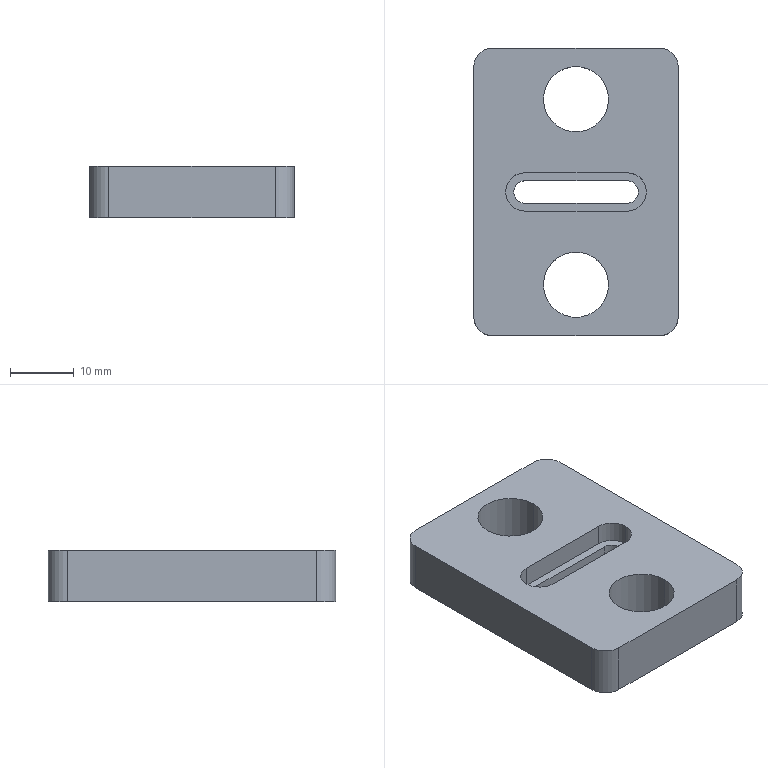Part | SolidWorks | features HoleWzd 2, ICE 2, Extrusion 1, Fillet 1 | 1 solid | 25 faces | box 32 x 45 x 8 mm | volume 9432 mm3 | cylinder 14 | plane 11 | commonest cylinder face diameters 6 x7 10.2 x4 3.5 x3
STEP:
#1=CARTESIAN_POINT('',(-5.1,-14.5,0.));
#2=VERTEX_POINT('',#1);
#3=CARTESIAN_POINT('',(5.1,-14.5,0.));
#4=VERTEX_POINT('',#3);
#5=CARTESIAN_POINT('',(0.,-14.5,0.));
#6=DIRECTION('',(0.,0.,1.));
#7=DIRECTION('',(1.,0.,0.));
#8=AXIS2_PLACEMENT_3D('',#5,#6,#7);
#9=CIRCLE('',#8,5.1);
#10=EDGE_CURVE('',#2,#4,#9,.T.);
#11=ORIENTED_EDGE('',*,*,#10,.F.);
#12=CARTESIAN_POINT('',(-5.1,-14.5,8.));
#13=VERTEX_POINT('',#12);
#14=CARTESIAN_POINT('',(-5.1,-14.5,8.));
#15=DIRECTION('',(0.,0.,1.));
#16=VECTOR('',#15,1000.);
#17=LINE('',#14,#16);
#18=EDGE_CURVE('',#2,#13,#17,.T.);
#19=ORIENTED_EDGE('',*,*,#18,.T.);
#20=CARTESIAN_POINT('',(5.1,-14.5,8.));
#21=VERTEX_POINT('',#20);
#22=CARTESIAN_POINT('',(0.,-14.5,8.));
#23=DIRECTION('',(0.,0.,1.));
#24=DIRECTION('',(1.,0.,0.));
#25=AXIS2_PLACEMENT_3D('',#22,#23,#24);
#26=CIRCLE('',#25,5.1);
#27=EDGE_CURVE('',#13,#21,#26,.T.);
#28=ORIENTED_EDGE('',*,*,#27,.T.);
#29=CARTESIAN_POINT('',(5.1,-14.5,8.));
#30=DIRECTION('',(0.,0.,1.));
#31=VECTOR('',#30,1000.);
#32=LINE('',#29,#31);
#33=EDGE_CURVE('',#4,#21,#32,.T.);
#34=ORIENTED_EDGE('',*,*,#33,.F.);
#35=EDGE_LOOP('',(#11,#19,#28,#34));
#36=FACE_OUTER_BOUND('',#35,.T.);
#37=CARTESIAN_POINT('',(0.,-14.5,8.));
#38=DIRECTION('',(0.,0.,1.));
#39=DIRECTION('',(1.,0.,0.));
#40=AXIS2_PLACEMENT_3D('',#37,#38,#39);
#41=CYLINDRICAL_SURFACE('',#40,5.1);
#42=ADVANCED_FACE('',(#36),#41,.F.);
#43=CARTESIAN_POINT('',(-5.1,14.5,0.));
#44=VERTEX_POINT('',#43);
#45=CARTESIAN_POINT('',(5.1,14.5,0.));
#46=VERTEX_POINT('',#45);
#47=CARTESIAN_POINT('',(0.,14.5,0.));
#48=DIRECTION('',(0.,0.,1.));
#49=DIRECTION('',(1.,0.,0.));
#50=AXIS2_PLACEMENT_3D('',#47,#48,#49);
#51=CIRCLE('',#50,5.1);
#52=EDGE_CURVE('',#44,#46,#51,.T.);
#53=ORIENTED_EDGE('',*,*,#52,.F.);
#54=CARTESIAN_POINT('',(-5.1,14.5,8.));
#55=VERTEX_POINT('',#54);
#56=CARTESIAN_POINT('',(-5.1,14.5,8.));
#57=DIRECTION('',(0.,0.,1.));
#58=VECTOR('',#57,1000.);
#59=LINE('',#56,#58);
#60=EDGE_CURVE('',#44,#55,#59,.T.);
#61=ORIENTED_EDGE('',*,*,#60,.T.);
#62=CARTESIAN_POINT('',(5.1,14.5,8.));
#63=VERTEX_POINT('',#62);
#64=CARTESIAN_POINT('',(0.,14.5,8.));
#65=DIRECTION('',(0.,0.,1.));
#66=DIRECTION('',(1.,0.,0.));
#67=AXIS2_PLACEMENT_3D('',#64,#65,#66);
#68=CIRCLE('',#67,5.1);
#69=EDGE_CURVE('',#55,#63,#68,.T.);
#70=ORIENTED_EDGE('',*,*,#69,.T.);
#71=CARTESIAN_POINT('',(5.1,14.5,8.));
#72=DIRECTION('',(0.,0.,1.));
#73=VECTOR('',#72,1000.);
#74=LINE('',#71,#73);
#75=EDGE_CURVE('',#46,#63,#74,.T.);
#76=ORIENTED_EDGE('',*,*,#75,.F.);
#77=EDGE_LOOP('',(#53,#61,#70,#76));
#78=FACE_OUTER_BOUND('',#77,.T.);
#79=CARTESIAN_POINT('',(0.,14.5,8.));
#80=DIRECTION('',(0.,0.,1.));
#81=DIRECTION('',(1.,0.,0.));
#82=AXIS2_PLACEMENT_3D('',#79,#80,#81);
#83=CYLINDRICAL_SURFACE('',#82,5.1);
#84=ADVANCED_FACE('',(#78),#83,.F.);
#85=CARTESIAN_POINT('',(11.,0.,4.7));
#86=VERTEX_POINT('',#85);
#87=CARTESIAN_POINT('',(8.,3.,4.7));
#88=VERTEX_POINT('',#87);
#89=CARTESIAN_POINT('',(8.,0.,4.7));
#90=DIRECTION('',(0.,0.,1.));
#91=DIRECTION('',(1.,0.,0.));
#92=AXIS2_PLACEMENT_3D('',#89,#90,#91);
#93=CIRCLE('',#92,3.);
#94=EDGE_CURVE('',#86,#88,#93,.T.);
#95=ORIENTED_EDGE('',*,*,#94,.F.);
#96=CARTESIAN_POINT('',(11.,0.,8.));
#97=VERTEX_POINT('',#96);
#98=CARTESIAN_POINT('',(11.,0.,4.7));
#99=DIRECTION('',(0.,0.,1.));
#100=VECTOR('',#99,1000.);
#101=LINE('',#98,#100);
#102=EDGE_CURVE('',#86,#97,#101,.T.);
#103=ORIENTED_EDGE('',*,*,#102,.T.);
#104=CARTESIAN_POINT('',(8.,3.,8.));
#105=VERTEX_POINT('',#104);
#106=CARTESIAN_POINT('',(8.,0.,8.));
#107=DIRECTION('',(0.,0.,1.));
#108=DIRECTION('',(1.,0.,0.));
#109=AXIS2_PLACEMENT_3D('',#106,#107,#108);
#110=CIRCLE('',#109,3.);
#111=EDGE_CURVE('',#97,#105,#110,.T.);
#112=ORIENTED_EDGE('',*,*,#111,.T.);
#113=CARTESIAN_POINT('',(8.,3.,4.7));
#114=DIRECTION('',(0.,0.,1.));
#115=VECTOR('',#114,1000.);
#116=LINE('',#113,#115);
#117=EDGE_CURVE('',#88,#105,#116,.T.);
#118=ORIENTED_EDGE('',*,*,#117,.F.);
#119=EDGE_LOOP('',(#95,#103,#112,#118));
#120=FACE_OUTER_BOUND('',#119,.T.);
#121=CARTESIAN_POINT('',(8.,0.,4.7));
#122=DIRECTION('',(0.,0.,1.));
#123=DIRECTION('',(1.,0.,0.));
#124=AXIS2_PLACEMENT_3D('',#121,#122,#123);
#125=CYLINDRICAL_SURFACE('',#124,3.);
#126=ADVANCED_FACE('',(#120),#125,.F.);
#127=CARTESIAN_POINT('',(9.75,0.,0.));
#128=VERTEX_POINT('',#127);
#129=CARTESIAN_POINT('',(8.,1.75,0.));
#130=VERTEX_POINT('',#129);
#131=CARTESIAN_POINT('',(8.,0.,0.));
#132=DIRECTION('',(0.,0.,1.));
#133=DIRECTION('',(1.,0.,0.));
#134=AXIS2_PLACEMENT_3D('',#131,#132,#133);
#135=CIRCLE('',#134,1.75);
#136=EDGE_CURVE('',#128,#130,#135,.T.);
#137=ORIENTED_EDGE('',*,*,#136,.F.);
#138=CARTESIAN_POINT('',(9.75,0.,4.7));
#139=VERTEX_POINT('',#138);
#140=CARTESIAN_POINT('',(9.75,0.,0.));
#141=DIRECTION('',(0.,0.,1.));
#142=VECTOR('',#141,1000.);
#143=LINE('',#140,#142);
#144=EDGE_CURVE('',#128,#139,#143,.T.);
#145=ORIENTED_EDGE('',*,*,#144,.T.);
#146=CARTESIAN_POINT('',(8.,1.75,4.7));
#147=VERTEX_POINT('',#146);
#148=CARTESIAN_POINT('',(8.,0.,4.7));
#149=DIRECTION('',(0.,0.,-1.));
#150=DIRECTION('',(1.,0.,0.));
#151=AXIS2_PLACEMENT_3D('',#148,#149,#150);
#152=CIRCLE('',#151,1.75);
#153=EDGE_CURVE('',#147,#139,#152,.T.);
#154=ORIENTED_EDGE('',*,*,#153,.F.);
#155=CARTESIAN_POINT('',(8.,1.75,0.));
#156=DIRECTION('',(0.,0.,1.));
#157=VECTOR('',#156,1000.);
#158=LINE('',#155,#157);
#159=EDGE_CURVE('',#130,#147,#158,.T.);
#160=ORIENTED_EDGE('',*,*,#159,.F.);
#161=EDGE_LOOP('',(#137,#145,#154,#160));
#162=FACE_OUTER_BOUND('',#161,.T.);
#163=CARTESIAN_POINT('',(8.,0.,0.));
#164=DIRECTION('',(0.,0.,1.));
#165=DIRECTION('',(1.,0.,0.));
#166=AXIS2_PLACEMENT_3D('',#163,#164,#165);
#167=CYLINDRICAL_SURFACE('',#166,1.75);
#168=ADVANCED_FACE('',(#162),#167,.F.);
#169=CARTESIAN_POINT('',(-8.,-1.75,4.7));
#170=VERTEX_POINT('',#169);
#171=CARTESIAN_POINT('',(-8.,1.75,4.7));
#172=VERTEX_POINT('',#171);
#173=CARTESIAN_POINT('',(-8.,0.,4.7));
#174=DIRECTION('',(0.,0.,-1.));
#175=DIRECTION('',(1.,0.,0.));
#176=AXIS2_PLACEMENT_3D('',#173,#174,#175);
#177=CIRCLE('',#176,1.75);
#178=EDGE_CURVE('',#170,#172,#177,.T.);
#179=ORIENTED_EDGE('',*,*,#178,.F.);
#180=CARTESIAN_POINT('',(-8.,-1.75,0.));
#181=VERTEX_POINT('',#180);
#182=CARTESIAN_POINT('',(-8.,-1.75,0.));
#183=DIRECTION('',(0.,0.,1.));
#184=VECTOR('',#183,1000.);
#185=LINE('',#182,#184);
#186=EDGE_CURVE('',#181,#170,#185,.T.);
#187=ORIENTED_EDGE('',*,*,#186,.F.);
#188=CARTESIAN_POINT('',(-8.,1.75,0.));
#189=VERTEX_POINT('',#188);
#190=CARTESIAN_POINT('',(-8.,0.,0.));
#191=DIRECTION('',(0.,0.,1.));
#192=DIRECTION('',(1.,0.,0.));
#193=AXIS2_PLACEMENT_3D('',#190,#191,#192);
#194=CIRCLE('',#193,1.75);
#195=EDGE_CURVE('',#189,#181,#194,.T.);
#196=ORIENTED_EDGE('',*,*,#195,.F.);
#197=CARTESIAN_POINT('',(-8.,1.75,0.));
#198=DIRECTION('',(0.,0.,1.));
#199=VECTOR('',#198,1000.);
#200=LINE('',#197,#199);
#201=EDGE_CURVE('',#189,#172,#200,.T.);
#202=ORIENTED_EDGE('',*,*,#201,.T.);
#203=EDGE_LOOP('',(#179,#187,#196,#202));
#204=FACE_OUTER_BOUND('',#203,.T.);
#205=CARTESIAN_POINT('',(-8.,0.,0.));
#206=DIRECTION('',(0.,0.,1.));
#207=DIRECTION('',(1.,0.,0.));
#208=AXIS2_PLACEMENT_3D('',#205,#206,#207);
#209=CYLINDRICAL_SURFACE('',#208,1.75);
#210=ADVANCED_FACE('',(#204),#209,.F.);
#211=CARTESIAN_POINT('',(-8.,1.75,4.7));
#212=DIRECTION('',(1.,0.,0.));
#213=VECTOR('',#212,1000.);
#214=LINE('',#211,#213);
#215=EDGE_CURVE('',#172,#147,#214,.T.);
#216=ORIENTED_EDGE('',*,*,#215,.F.);
#217=ORIENTED_EDGE('',*,*,#201,.F.);
#218=CARTESIAN_POINT('',(-8.,1.75,0.));
#219=DIRECTION('',(-1.,0.,0.));
#220=VECTOR('',#219,1000.);
#221=LINE('',#218,#220);
#222=EDGE_CURVE('',#130,#189,#221,.T.);
#223=ORIENTED_EDGE('',*,*,#222,.F.);
#224=ORIENTED_EDGE('',*,*,#159,.T.);
#225=EDGE_LOOP('',(#216,#217,#223,#224));
#226=FACE_OUTER_BOUND('',#225,.T.);
#227=CARTESIAN_POINT('',(-8.,1.75,0.));
#228=DIRECTION('',(0.,1.,0.));
#229=DIRECTION('',(0.,0.,1.));
#230=AXIS2_PLACEMENT_3D('',#227,#228,#229);
#231=PLANE('',#230);
#232=ADVANCED_FACE('',(#226),#231,.F.);
#233=ORIENTED_EDGE('',*,*,#144,.F.);
#234=CARTESIAN_POINT('',(8.,-1.75,0.));
#235=VERTEX_POINT('',#234);
#236=CARTESIAN_POINT('',(8.,0.,0.));
#237=DIRECTION('',(0.,0.,1.));
#238=DIRECTION('',(1.,0.,0.));
#239=AXIS2_PLACEMENT_3D('',#236,#237,#238);
#240=CIRCLE('',#239,1.75);
#241=EDGE_CURVE('',#235,#128,#240,.T.);
#242=ORIENTED_EDGE('',*,*,#241,.F.);
#243=CARTESIAN_POINT('',(8.,-1.75,4.7));
#244=VERTEX_POINT('',#243);
#245=CARTESIAN_POINT('',(8.,-1.75,0.));
#246=DIRECTION('',(0.,0.,1.));
#247=VECTOR('',#246,1000.);
#248=LINE('',#245,#247);
#249=EDGE_CURVE('',#235,#244,#248,.T.);
#250=ORIENTED_EDGE('',*,*,#249,.T.);
#251=CARTESIAN_POINT('',(8.,0.,4.7));
#252=DIRECTION('',(0.,0.,-1.));
#253=DIRECTION('',(1.,0.,0.));
#254=AXIS2_PLACEMENT_3D('',#251,#252,#253);
#255=CIRCLE('',#254,1.75);
#256=EDGE_CURVE('',#139,#244,#255,.T.);
#257=ORIENTED_EDGE('',*,*,#256,.F.);
#258=EDGE_LOOP('',(#233,#242,#250,#257));
#259=FACE_OUTER_BOUND('',#258,.T.);
#260=CARTESIAN_POINT('',(8.,0.,0.));
#261=DIRECTION('',(0.,0.,1.));
#262=DIRECTION('',(1.,0.,0.));
#263=AXIS2_PLACEMENT_3D('',#260,#261,#262);
#264=CYLINDRICAL_SURFACE('',#263,1.75);
#265=ADVANCED_FACE('',(#259),#264,.F.);
#266=CARTESIAN_POINT('',(-8.,-1.75,4.7));
#267=DIRECTION('',(-1.,0.,0.));
#268=VECTOR('',#267,1000.);
#269=LINE('',#266,#268);
#270=EDGE_CURVE('',#244,#170,#269,.T.);
#271=ORIENTED_EDGE('',*,*,#270,.F.);
#272=ORIENTED_EDGE('',*,*,#249,.F.);
#273=CARTESIAN_POINT('',(-8.,-1.75,0.));
#274=DIRECTION('',(1.,0.,0.));
#275=VECTOR('',#274,1000.);
#276=LINE('',#273,#275);
#277=EDGE_CURVE('',#181,#235,#276,.T.);
#278=ORIENTED_EDGE('',*,*,#277,.F.);
#279=ORIENTED_EDGE('',*,*,#186,.T.);
#280=EDGE_LOOP('',(#271,#272,#278,#279));
#281=FACE_OUTER_BOUND('',#280,.T.);
#282=CARTESIAN_POINT('',(-8.,-1.75,0.));
#283=DIRECTION('',(0.,-1.,0.));
#284=DIRECTION('',(0.,0.,-1.));
#285=AXIS2_PLACEMENT_3D('',#282,#283,#284);
#286=PLANE('',#285);
#287=ADVANCED_FACE('',(#281),#286,.F.);
#288=CARTESIAN_POINT('',(-16.,19.5,8.));
#289=VERTEX_POINT('',#288);
#290=CARTESIAN_POINT('',(-16.,-19.5,8.));
#291=VERTEX_POINT('',#290);
#292=CARTESIAN_POINT('',(-16.,-22.5,8.));
#293=DIRECTION('',(0.,-1.,0.));
#294=VECTOR('',#293,1000.);
#295=LINE('',#292,#294);
#296=EDGE_CURVE('',#289,#291,#295,.T.);
#297=ORIENTED_EDGE('',*,*,#296,.F.);
#298=CARTESIAN_POINT('',(-16.,19.5,0.));
#299=VERTEX_POINT('',#298);
#300=CARTESIAN_POINT('',(-16.,19.5,8.));
#301=DIRECTION('',(0.,0.,-1.));
#302=VECTOR('',#301,1000.);
#303=LINE('',#300,#302);
#304=EDGE_CURVE('',#289,#299,#303,.T.);
#305=ORIENTED_EDGE('',*,*,#304,.T.);
#306=CARTESIAN_POINT('',(-16.,-19.5,0.));
#307=VERTEX_POINT('',#306);
#308=CARTESIAN_POINT('',(-16.,-22.5,0.));
#309=DIRECTION('',(0.,-1.,0.));
#310=VECTOR('',#309,1000.);
#311=LINE('',#308,#310);
#312=EDGE_CURVE('',#299,#307,#311,.T.);
#313=ORIENTED_EDGE('',*,*,#312,.T.);
#314=CARTESIAN_POINT('',(-16.,-19.5,8.));
#315=DIRECTION('',(0.,0.,1.));
#316=VECTOR('',#315,1000.);
#317=LINE('',#314,#316);
#318=EDGE_CURVE('',#307,#291,#317,.T.);
#319=ORIENTED_EDGE('',*,*,#318,.T.);
#320=EDGE_LOOP('',(#297,#305,#313,#319));
#321=FACE_OUTER_BOUND('',#320,.T.);
#322=CARTESIAN_POINT('',(-16.,-22.5,8.));
#323=DIRECTION('',(1.,0.,0.));
#324=DIRECTION('',(0.,0.,-1.));
#325=AXIS2_PLACEMENT_3D('',#322,#323,#324);
#326=PLANE('',#325);
#327=ADVANCED_FACE('',(#321),#326,.F.);
#328=CARTESIAN_POINT('',(-13.,-22.5,0.));
#329=VERTEX_POINT('',#328);
#330=CARTESIAN_POINT('',(13.,-22.5,0.));
#331=VERTEX_POINT('',#330);
#332=CARTESIAN_POINT('',(16.,-22.5,0.));
#333=DIRECTION('',(1.,0.,0.));
#334=VECTOR('',#333,1000.);
#335=LINE('',#332,#334);
#336=EDGE_CURVE('',#329,#331,#335,.T.);
#337=ORIENTED_EDGE('',*,*,#336,.T.);
#338=CARTESIAN_POINT('',(13.,-22.5,8.));
#339=VERTEX_POINT('',#338);
#340=CARTESIAN_POINT('',(13.,-22.5,8.));
#341=DIRECTION('',(0.,0.,1.));
#342=VECTOR('',#341,1000.);
#343=LINE('',#340,#342);
#344=EDGE_CURVE('',#331,#339,#343,.T.);
#345=ORIENTED_EDGE('',*,*,#344,.T.);
#346=CARTESIAN_POINT('',(-13.,-22.5,8.));
#347=VERTEX_POINT('',#346);
#348=CARTESIAN_POINT('',(16.,-22.5,8.));
#349=DIRECTION('',(1.,0.,0.));
#350=VECTOR('',#349,1000.);
#351=LINE('',#348,#350);
#352=EDGE_CURVE('',#347,#339,#351,.T.);
#353=ORIENTED_EDGE('',*,*,#352,.F.);
#354=CARTESIAN_POINT('',(-13.,-22.5,8.));
#355=DIRECTION('',(0.,0.,-1.));
#356=VECTOR('',#355,1000.);
#357=LINE('',#354,#356);
#358=EDGE_CURVE('',#347,#329,#357,.T.);
#359=ORIENTED_EDGE('',*,*,#358,.T.);
#360=EDGE_LOOP('',(#337,#345,#353,#359));
#361=FACE_OUTER_BOUND('',#360,.T.);
#362=CARTESIAN_POINT('',(16.,-22.5,8.));
#363=DIRECTION('',(0.,1.,0.));
#364=DIRECTION('',(-1.,0.,0.));
#365=AXIS2_PLACEMENT_3D('',#362,#363,#364);
#366=PLANE('',#365);
#367=ADVANCED_FACE('',(#361),#366,.F.);
#368=CARTESIAN_POINT('',(16.,-19.5,0.));
#369=VERTEX_POINT('',#368);
#370=CARTESIAN_POINT('',(16.,19.5,0.));
#371=VERTEX_POINT('',#370);
#372=CARTESIAN_POINT('',(16.,-22.5,0.));
#373=DIRECTION('',(0.,1.,0.));
#374=VECTOR('',#373,1000.);
#375=LINE('',#372,#374);
#376=EDGE_CURVE('',#369,#371,#375,.T.);
#377=ORIENTED_EDGE('',*,*,#376,.T.);
#378=CARTESIAN_POINT('',(16.,19.5,8.));
#379=VERTEX_POINT('',#378);
#380=CARTESIAN_POINT('',(16.,19.5,8.));
#381=DIRECTION('',(0.,0.,1.));
#382=VECTOR('',#381,1000.);
#383=LINE('',#380,#382);
#384=EDGE_CURVE('',#371,#379,#383,.T.);
#385=ORIENTED_EDGE('',*,*,#384,.T.);
#386=CARTESIAN_POINT('',(16.,-19.5,8.));
#387=VERTEX_POINT('',#386);
#388=CARTESIAN_POINT('',(16.,-22.5,8.));
#389=DIRECTION('',(0.,1.,0.));
#390=VECTOR('',#389,1000.);
#391=LINE('',#388,#390);
#392=EDGE_CURVE('',#387,#379,#391,.T.);
#393=ORIENTED_EDGE('',*,*,#392,.F.);
#394=CARTESIAN_POINT('',(16.,-19.5,8.));
#395=DIRECTION('',(0.,0.,-1.));
#396=VECTOR('',#395,1000.);
#397=LINE('',#394,#396);
#398=EDGE_CURVE('',#387,#369,#397,.T.);
#399=ORIENTED_EDGE('',*,*,#398,.T.);
#400=EDGE_LOOP('',(#377,#385,#393,#399));
#401=FACE_OUTER_BOUND('',#400,.T.);
#402=CARTESIAN_POINT('',(16.,-22.5,8.));
#403=DIRECTION('',(-1.,0.,0.));
#404=DIRECTION('',(0.,0.,1.));
#405=AXIS2_PLACEMENT_3D('',#402,#403,#404);
#406=PLANE('',#405);
#407=ADVANCED_FACE('',(#401),#406,.F.);
#408=CARTESIAN_POINT('',(13.,22.5,0.));
#409=VERTEX_POINT('',#408);
#410=CARTESIAN_POINT('',(-13.,22.5,0.));
#411=VERTEX_POINT('',#410);
#412=CARTESIAN_POINT('',(16.,22.5,0.));
#413=DIRECTION('',(-1.,0.,0.));
#414=VECTOR('',#413,1000.);
#415=LINE('',#412,#414);
#416=EDGE_CURVE('',#409,#411,#415,.T.);
#417=ORIENTED_EDGE('',*,*,#416,.T.);
#418=CARTESIAN_POINT('',(-13.,22.5,8.));
#419=VERTEX_POINT('',#418);
#420=CARTESIAN_POINT('',(-13.,22.5,8.));
#421=DIRECTION('',(0.,0.,1.));
#422=VECTOR('',#421,1000.);
#423=LINE('',#420,#422);
#424=EDGE_CURVE('',#411,#419,#423,.T.);
#425=ORIENTED_EDGE('',*,*,#424,.T.);
#426=CARTESIAN_POINT('',(13.,22.5,8.));
#427=VERTEX_POINT('',#426);
#428=CARTESIAN_POINT('',(16.,22.5,8.));
#429=DIRECTION('',(-1.,0.,0.));
#430=VECTOR('',#429,1000.);
#431=LINE('',#428,#430);
#432=EDGE_CURVE('',#427,#419,#431,.T.);
#433=ORIENTED_EDGE('',*,*,#432,.F.);
#434=CARTESIAN_POINT('',(13.,22.5,8.));
#435=DIRECTION('',(0.,0.,-1.));
#436=VECTOR('',#435,1000.);
#437=LINE('',#434,#436);
#438=EDGE_CURVE('',#427,#409,#437,.T.);
#439=ORIENTED_EDGE('',*,*,#438,.T.);
#440=EDGE_LOOP('',(#417,#425,#433,#439));
#441=FACE_OUTER_BOUND('',#440,.T.);
#442=CARTESIAN_POINT('',(16.,22.5,8.));
#443=DIRECTION('',(0.,-1.,0.));
#444=DIRECTION('',(1.,0.,0.));
#445=AXIS2_PLACEMENT_3D('',#442,#443,#444);
#446=PLANE('',#445);
#447=ADVANCED_FACE('',(#441),#446,.F.);
#448=CARTESIAN_POINT('',(0.,-14.5,8.));
#449=DIRECTION('',(0.,0.,1.));
#450=DIRECTION('',(1.,0.,0.));
#451=AXIS2_PLACEMENT_3D('',#448,#449,#450);
#452=CIRCLE('',#451,5.1);
#453=EDGE_CURVE('',#21,#13,#452,.T.);
#454=ORIENTED_EDGE('',*,*,#453,.F.);
#455=ORIENTED_EDGE('',*,*,#27,.F.);
#456=EDGE_LOOP('',(#454,#455));
#457=FACE_BOUND('',#456,.T.);
#458=CARTESIAN_POINT('',(0.,14.5,8.));
#459=DIRECTION('',(0.,0.,1.));
#460=DIRECTION('',(1.,0.,0.));
#461=AXIS2_PLACEMENT_3D('',#458,#459,#460);
#462=CIRCLE('',#461,5.1);
#463=EDGE_CURVE('',#63,#55,#462,.T.);
#464=ORIENTED_EDGE('',*,*,#463,.F.);
#465=ORIENTED_EDGE('',*,*,#69,.F.);
#466=EDGE_LOOP('',(#464,#465));
#467=FACE_BOUND('',#466,.T.);
#468=CARTESIAN_POINT('',(-8.,3.,8.));
#469=VERTEX_POINT('',#468);
#470=CARTESIAN_POINT('',(-8.,-3.,8.));
#471=VERTEX_POINT('',#470);
#472=CARTESIAN_POINT('',(-8.,0.,8.));
#473=DIRECTION('',(0.,0.,1.));
#474=DIRECTION('',(1.,0.,0.));
#475=AXIS2_PLACEMENT_3D('',#472,#473,#474);
#476=CIRCLE('',#475,3.);
#477=EDGE_CURVE('',#469,#471,#476,.T.);
#478=ORIENTED_EDGE('',*,*,#477,.F.);
#479=CARTESIAN_POINT('',(-8.,3.,8.));
#480=DIRECTION('',(-1.,0.,0.));
#481=VECTOR('',#480,1000.);
#482=LINE('',#479,#481);
#483=EDGE_CURVE('',#105,#469,#482,.T.);
#484=ORIENTED_EDGE('',*,*,#483,.F.);
#485=ORIENTED_EDGE('',*,*,#111,.F.);
#486=CARTESIAN_POINT('',(8.,-3.,8.));
#487=VERTEX_POINT('',#486);
#488=CARTESIAN_POINT('',(8.,0.,8.));
#489=DIRECTION('',(0.,0.,1.));
#490=DIRECTION('',(1.,0.,0.));
#491=AXIS2_PLACEMENT_3D('',#488,#489,#490);
#492=CIRCLE('',#491,3.);
#493=EDGE_CURVE('',#487,#97,#492,.T.);
#494=ORIENTED_EDGE('',*,*,#493,.F.);
#495=CARTESIAN_POINT('',(-8.,-3.,8.));
#496=DIRECTION('',(1.,0.,0.));
#497=VECTOR('',#496,1000.);
#498=LINE('',#495,#497);
#499=EDGE_CURVE('',#471,#487,#498,.T.);
#500=ORIENTED_EDGE('',*,*,#499,.F.);
#501=EDGE_LOOP('',(#478,#484,#485,#494,#500));
#502=FACE_BOUND('',#501,.T.);
#503=ORIENTED_EDGE('',*,*,#432,.T.);
#504=CARTESIAN_POINT('',(-13.,19.5,8.));
#505=DIRECTION('',(0.,0.,1.));
#506=DIRECTION('',(1.,0.,0.));
#507=AXIS2_PLACEMENT_3D('',#504,#505,#506);
#508=CIRCLE('',#507,3.);
#509=EDGE_CURVE('',#419,#289,#508,.T.);
#510=ORIENTED_EDGE('',*,*,#509,.T.);
#511=ORIENTED_EDGE('',*,*,#296,.T.);
#512=CARTESIAN_POINT('',(-13.,-19.5,8.));
#513=DIRECTION('',(0.,0.,1.));
#514=DIRECTION('',(1.,0.,0.));
#515=AXIS2_PLACEMENT_3D('',#512,#513,#514);
#516=CIRCLE('',#515,3.);
#517=EDGE_CURVE('',#291,#347,#516,.T.);
#518=ORIENTED_EDGE('',*,*,#517,.T.);
#519=ORIENTED_EDGE('',*,*,#352,.T.);
#520=CARTESIAN_POINT('',(13.,-19.5,8.));
#521=DIRECTION('',(0.,0.,1.));
#522=DIRECTION('',(1.,0.,0.));
#523=AXIS2_PLACEMENT_3D('',#520,#521,#522);
#524=CIRCLE('',#523,3.);
#525=EDGE_CURVE('',#339,#387,#524,.T.);
#526=ORIENTED_EDGE('',*,*,#525,.T.);
#527=ORIENTED_EDGE('',*,*,#392,.T.);
#528=CARTESIAN_POINT('',(13.,19.5,8.));
#529=DIRECTION('',(0.,0.,1.));
#530=DIRECTION('',(1.,0.,0.));
#531=AXIS2_PLACEMENT_3D('',#528,#529,#530);
#532=CIRCLE('',#531,3.);
#533=EDGE_CURVE('',#379,#427,#532,.T.);
#534=ORIENTED_EDGE('',*,*,#533,.T.);
#535=EDGE_LOOP('',(#503,#510,#511,#518,#519,#526,#527,#534));
#536=FACE_OUTER_BOUND('',#535,.T.);
#537=CARTESIAN_POINT('',(0.,0.,8.));
#538=DIRECTION('',(0.,0.,1.));
#539=DIRECTION('',(1.,0.,0.));
#540=AXIS2_PLACEMENT_3D('',#537,#538,#539);
#541=PLANE('',#540);
#542=ADVANCED_FACE('',(#457,#467,#502,#536),#541,.T.);
#543=CARTESIAN_POINT('',(0.,-14.5,0.));
#544=DIRECTION('',(0.,0.,1.));
#545=DIRECTION('',(1.,0.,0.));
#546=AXIS2_PLACEMENT_3D('',#543,#544,#545);
#547=CIRCLE('',#546,5.1);
#548=EDGE_CURVE('',#4,#2,#547,.T.);
#549=ORIENTED_EDGE('',*,*,#548,.T.);
#550=ORIENTED_EDGE('',*,*,#10,.T.);
#551=EDGE_LOOP('',(#549,#550));
#552=FACE_BOUND('',#551,.T.);
#553=CARTESIAN_POINT('',(0.,14.5,0.));
#554=DIRECTION('',(0.,0.,1.));
#555=DIRECTION('',(1.,0.,0.));
#556=AXIS2_PLACEMENT_3D('',#553,#554,#555);
#557=CIRCLE('',#556,5.1);
#558=EDGE_CURVE('',#46,#44,#557,.T.);
#559=ORIENTED_EDGE('',*,*,#558,.T.);
#560=ORIENTED_EDGE('',*,*,#52,.T.);
#561=EDGE_LOOP('',(#559,#560));
#562=FACE_BOUND('',#561,.T.);
#563=ORIENTED_EDGE('',*,*,#222,.T.);
#564=ORIENTED_EDGE('',*,*,#195,.T.);
#565=ORIENTED_EDGE('',*,*,#277,.T.);
#566=ORIENTED_EDGE('',*,*,#241,.T.);
#567=ORIENTED_EDGE('',*,*,#136,.T.);
#568=EDGE_LOOP('',(#563,#564,#565,#566,#567));
#569=FACE_BOUND('',#568,.T.);
#570=ORIENTED_EDGE('',*,*,#312,.F.);
#571=CARTESIAN_POINT('',(-13.,19.5,0.));
#572=DIRECTION('',(0.,0.,-1.));
#573=DIRECTION('',(1.,0.,0.));
#574=AXIS2_PLACEMENT_3D('',#571,#572,#573);
#575=CIRCLE('',#574,3.);
#576=EDGE_CURVE('',#299,#411,#575,.T.);
#577=ORIENTED_EDGE('',*,*,#576,.T.);
#578=ORIENTED_EDGE('',*,*,#416,.F.);
#579=CARTESIAN_POINT('',(13.,19.5,0.));
#580=DIRECTION('',(0.,0.,-1.));
#581=DIRECTION('',(1.,0.,0.));
#582=AXIS2_PLACEMENT_3D('',#579,#580,#581);
#583=CIRCLE('',#582,3.);
#584=EDGE_CURVE('',#409,#371,#583,.T.);
#585=ORIENTED_EDGE('',*,*,#584,.T.);
#586=ORIENTED_EDGE('',*,*,#376,.F.);
#587=CARTESIAN_POINT('',(13.,-19.5,0.));
#588=DIRECTION('',(0.,0.,-1.));
#589=DIRECTION('',(1.,0.,0.));
#590=AXIS2_PLACEMENT_3D('',#587,#588,#589);
#591=CIRCLE('',#590,3.);
#592=EDGE_CURVE('',#369,#331,#591,.T.);
#593=ORIENTED_EDGE('',*,*,#592,.T.);
#594=ORIENTED_EDGE('',*,*,#336,.F.);
#595=CARTESIAN_POINT('',(-13.,-19.5,0.));
#596=DIRECTION('',(0.,0.,-1.));
#597=DIRECTION('',(1.,0.,0.));
#598=AXIS2_PLACEMENT_3D('',#595,#596,#597);
#599=CIRCLE('',#598,3.);
#600=EDGE_CURVE('',#329,#307,#599,.T.);
#601=ORIENTED_EDGE('',*,*,#600,.T.);
#602=EDGE_LOOP('',(#570,#577,#578,#585,#586,#593,#594,#601));
#603=FACE_OUTER_BOUND('',#602,.T.);
#604=CARTESIAN_POINT('',(0.,0.,0.));
#605=DIRECTION('',(0.,0.,1.));
#606=DIRECTION('',(1.,0.,0.));
#607=AXIS2_PLACEMENT_3D('',#604,#605,#606);
#608=PLANE('',#607);
#609=ADVANCED_FACE('',(#552,#562,#569,#603),#608,.F.);
#610=CARTESIAN_POINT('',(-8.,3.,4.7));
#611=VERTEX_POINT('',#610);
#612=CARTESIAN_POINT('',(-8.,-3.,4.7));
#613=VERTEX_POINT('',#612);
#614=CARTESIAN_POINT('',(-8.,0.,4.7));
#615=DIRECTION('',(0.,0.,1.));
#616=DIRECTION('',(1.,0.,0.));
#617=AXIS2_PLACEMENT_3D('',#614,#615,#616);
#618=CIRCLE('',#617,3.);
#619=EDGE_CURVE('',#611,#613,#618,.T.);
#620=ORIENTED_EDGE('',*,*,#619,.T.);
#621=CARTESIAN_POINT('',(8.,-3.,4.7));
#622=VERTEX_POINT('',#621);
#623=CARTESIAN_POINT('',(-8.,-3.,4.7));
#624=DIRECTION('',(1.,0.,0.));
#625=VECTOR('',#624,1000.);
#626=LINE('',#623,#625);
#627=EDGE_CURVE('',#613,#622,#626,.T.);
#628=ORIENTED_EDGE('',*,*,#627,.T.);
#629=CARTESIAN_POINT('',(8.,0.,4.7));
#630=DIRECTION('',(0.,0.,1.));
#631=DIRECTION('',(1.,0.,0.));
#632=AXIS2_PLACEMENT_3D('',#629,#630,#631);
#633=CIRCLE('',#632,3.);
#634=EDGE_CURVE('',#622,#86,#633,.T.);
#635=ORIENTED_EDGE('',*,*,#634,.T.);
#636=ORIENTED_EDGE('',*,*,#94,.T.);
#637=CARTESIAN_POINT('',(-8.,3.,4.7));
#638=DIRECTION('',(-1.,0.,0.));
#639=VECTOR('',#638,1000.);
#640=LINE('',#637,#639);
#641=EDGE_CURVE('',#88,#611,#640,.T.);
#642=ORIENTED_EDGE('',*,*,#641,.T.);
#643=EDGE_LOOP('',(#620,#628,#635,#636,#642));
#644=FACE_OUTER_BOUND('',#643,.T.);
#645=ORIENTED_EDGE('',*,*,#178,.T.);
#646=ORIENTED_EDGE('',*,*,#215,.T.);
#647=ORIENTED_EDGE('',*,*,#153,.T.);
#648=ORIENTED_EDGE('',*,*,#256,.T.);
#649=ORIENTED_EDGE('',*,*,#270,.T.);
#650=EDGE_LOOP('',(#645,#646,#647,#648,#649));
#651=FACE_BOUND('',#650,.T.);
#652=CARTESIAN_POINT('',(-8.,0.,4.7));
#653=DIRECTION('',(0.,0.,1.));
#654=DIRECTION('',(1.,0.,0.));
#655=AXIS2_PLACEMENT_3D('',#652,#653,#654);
#656=PLANE('',#655);
#657=ADVANCED_FACE('',(#644,#651),#656,.T.);
#658=ORIENTED_EDGE('',*,*,#477,.T.);
#659=CARTESIAN_POINT('',(-8.,-3.,4.7));
#660=DIRECTION('',(0.,0.,1.));
#661=VECTOR('',#660,1000.);
#662=LINE('',#659,#661);
#663=EDGE_CURVE('',#613,#471,#662,.T.);
#664=ORIENTED_EDGE('',*,*,#663,.F.);
#665=ORIENTED_EDGE('',*,*,#619,.F.);
#666=CARTESIAN_POINT('',(-8.,3.,4.7));
#667=DIRECTION('',(0.,0.,1.));
#668=VECTOR('',#667,1000.);
#669=LINE('',#666,#668);
#670=EDGE_CURVE('',#611,#469,#669,.T.);
#671=ORIENTED_EDGE('',*,*,#670,.T.);
#672=EDGE_LOOP('',(#658,#664,#665,#671));
#673=FACE_OUTER_BOUND('',#672,.T.);
#674=CARTESIAN_POINT('',(-8.,0.,4.7));
#675=DIRECTION('',(0.,0.,1.));
#676=DIRECTION('',(1.,0.,0.));
#677=AXIS2_PLACEMENT_3D('',#674,#675,#676);
#678=CYLINDRICAL_SURFACE('',#677,3.);
#679=ADVANCED_FACE('',(#673),#678,.F.);
#680=ORIENTED_EDGE('',*,*,#483,.T.);
#681=ORIENTED_EDGE('',*,*,#670,.F.);
#682=ORIENTED_EDGE('',*,*,#641,.F.);
#683=ORIENTED_EDGE('',*,*,#117,.T.);
#684=EDGE_LOOP('',(#680,#681,#682,#683));
#685=FACE_OUTER_BOUND('',#684,.T.);
#686=CARTESIAN_POINT('',(-8.,3.,4.7));
#687=DIRECTION('',(0.,1.,0.));
#688=DIRECTION('',(0.,0.,1.));
#689=AXIS2_PLACEMENT_3D('',#686,#687,#688);
#690=PLANE('',#689);
#691=ADVANCED_FACE('',(#685),#690,.F.);
#692=ORIENTED_EDGE('',*,*,#102,.F.);
#693=ORIENTED_EDGE('',*,*,#634,.F.);
#694=CARTESIAN_POINT('',(8.,-3.,4.7));
#695=DIRECTION('',(0.,0.,1.));
#696=VECTOR('',#695,1000.);
#697=LINE('',#694,#696);
#698=EDGE_CURVE('',#622,#487,#697,.T.);
#699=ORIENTED_EDGE('',*,*,#698,.T.);
#700=ORIENTED_EDGE('',*,*,#493,.T.);
#701=EDGE_LOOP('',(#692,#693,#699,#700));
#702=FACE_OUTER_BOUND('',#701,.T.);
#703=CARTESIAN_POINT('',(8.,0.,4.7));
#704=DIRECTION('',(0.,0.,1.));
#705=DIRECTION('',(1.,0.,0.));
#706=AXIS2_PLACEMENT_3D('',#703,#704,#705);
#707=CYLINDRICAL_SURFACE('',#706,3.);
#708=ADVANCED_FACE('',(#702),#707,.F.);
#709=ORIENTED_EDGE('',*,*,#499,.T.);
#710=ORIENTED_EDGE('',*,*,#698,.F.);
#711=ORIENTED_EDGE('',*,*,#627,.F.);
#712=ORIENTED_EDGE('',*,*,#663,.T.);
#713=EDGE_LOOP('',(#709,#710,#711,#712));
#714=FACE_OUTER_BOUND('',#713,.T.);
#715=CARTESIAN_POINT('',(-8.,-3.,4.7));
#716=DIRECTION('',(0.,-1.,0.));
#717=DIRECTION('',(0.,0.,-1.));
#718=AXIS2_PLACEMENT_3D('',#715,#716,#717);
#719=PLANE('',#718);
#720=ADVANCED_FACE('',(#714),#719,.F.);
#721=ORIENTED_EDGE('',*,*,#509,.F.);
#722=ORIENTED_EDGE('',*,*,#424,.F.);
#723=ORIENTED_EDGE('',*,*,#576,.F.);
#724=ORIENTED_EDGE('',*,*,#304,.F.);
#725=EDGE_LOOP('',(#721,#722,#723,#724));
#726=FACE_OUTER_BOUND('',#725,.T.);
#727=CARTESIAN_POINT('',(-13.,19.5,8.));
#728=DIRECTION('',(0.,0.,-1.));
#729=DIRECTION('',(-1.,0.,0.));
#730=AXIS2_PLACEMENT_3D('',#727,#728,#729);
#731=CYLINDRICAL_SURFACE('',#730,3.);
#732=ADVANCED_FACE('',(#726),#731,.T.);
#733=ORIENTED_EDGE('',*,*,#533,.F.);
#734=ORIENTED_EDGE('',*,*,#384,.F.);
#735=ORIENTED_EDGE('',*,*,#584,.F.);
#736=ORIENTED_EDGE('',*,*,#438,.F.);
#737=EDGE_LOOP('',(#733,#734,#735,#736));
#738=FACE_OUTER_BOUND('',#737,.T.);
#739=CARTESIAN_POINT('',(13.,19.5,8.));
#740=DIRECTION('',(0.,0.,-1.));
#741=DIRECTION('',(-1.,0.,0.));
#742=AXIS2_PLACEMENT_3D('',#739,#740,#741);
#743=CYLINDRICAL_SURFACE('',#742,3.);
#744=ADVANCED_FACE('',(#738),#743,.T.);
#745=ORIENTED_EDGE('',*,*,#525,.F.);
#746=ORIENTED_EDGE('',*,*,#344,.F.);
#747=ORIENTED_EDGE('',*,*,#592,.F.);
#748=ORIENTED_EDGE('',*,*,#398,.F.);
#749=EDGE_LOOP('',(#745,#746,#747,#748));
#750=FACE_OUTER_BOUND('',#749,.T.);
#751=CARTESIAN_POINT('',(13.,-19.5,8.));
#752=DIRECTION('',(0.,0.,-1.));
#753=DIRECTION('',(-1.,0.,0.));
#754=AXIS2_PLACEMENT_3D('',#751,#752,#753);
#755=CYLINDRICAL_SURFACE('',#754,3.);
#756=ADVANCED_FACE('',(#750),#755,.T.);
#757=ORIENTED_EDGE('',*,*,#517,.F.);
#758=ORIENTED_EDGE('',*,*,#318,.F.);
#759=ORIENTED_EDGE('',*,*,#600,.F.);
#760=ORIENTED_EDGE('',*,*,#358,.F.);
#761=EDGE_LOOP('',(#757,#758,#759,#760));
#762=FACE_OUTER_BOUND('',#761,.T.);
#763=CARTESIAN_POINT('',(-13.,-19.5,8.));
#764=DIRECTION('',(0.,0.,-1.));
#765=DIRECTION('',(-1.,0.,0.));
#766=AXIS2_PLACEMENT_3D('',#763,#764,#765);
#767=CYLINDRICAL_SURFACE('',#766,3.);
#768=ADVANCED_FACE('',(#762),#767,.T.);
#769=ORIENTED_EDGE('',*,*,#60,.F.);
#770=ORIENTED_EDGE('',*,*,#558,.F.);
#771=ORIENTED_EDGE('',*,*,#75,.T.);
#772=ORIENTED_EDGE('',*,*,#463,.T.);
#773=EDGE_LOOP('',(#769,#770,#771,#772));
#774=FACE_OUTER_BOUND('',#773,.T.);
#775=CARTESIAN_POINT('',(0.,14.5,8.));
#776=DIRECTION('',(0.,0.,1.));
#777=DIRECTION('',(1.,0.,0.));
#778=AXIS2_PLACEMENT_3D('',#775,#776,#777);
#779=CYLINDRICAL_SURFACE('',#778,5.1);
#780=ADVANCED_FACE('',(#774),#779,.F.);
#781=ORIENTED_EDGE('',*,*,#18,.F.);
#782=ORIENTED_EDGE('',*,*,#548,.F.);
#783=ORIENTED_EDGE('',*,*,#33,.T.);
#784=ORIENTED_EDGE('',*,*,#453,.T.);
#785=EDGE_LOOP('',(#781,#782,#783,#784));
#786=FACE_OUTER_BOUND('',#785,.T.);
#787=CARTESIAN_POINT('',(0.,-14.5,8.));
#788=DIRECTION('',(0.,0.,1.));
#789=DIRECTION('',(1.,0.,0.));
#790=AXIS2_PLACEMENT_3D('',#787,#788,#789);
#791=CYLINDRICAL_SURFACE('',#790,5.1);
#792=ADVANCED_FACE('',(#786),#791,.F.);
#793=CLOSED_SHELL('',(#42,#84,#126,#168,#210,#232,#265,#287,#327,#367,#407,#447,#542,#609,#657,#679,#691,#708,#720,#732,#744,#756,#768,#780,#792));
#794=MANIFOLD_SOLID_BREP('',#793);
#795=CARTESIAN_POINT('',(0.,0.,0.));
#796=DIRECTION('',(0.,0.,1.));
#797=DIRECTION('',(1.,0.,0.));
#798=AXIS2_PLACEMENT_3D('',#795,#796,#797);
#799=(LENGTH_UNIT()NAMED_UNIT(*)SI_UNIT(.MILLI.,.METRE.));
#800=UNCERTAINTY_MEASURE_WITH_UNIT(LENGTH_MEASURE(0.00001),#799,'','');
#801=(NAMED_UNIT(*)PLANE_ANGLE_UNIT()SI_UNIT($,.RADIAN.));
#802=(NAMED_UNIT(*)SI_UNIT($,.STERADIAN.)SOLID_ANGLE_UNIT());
#803=(GEOMETRIC_REPRESENTATION_CONTEXT(3)GLOBAL_UNCERTAINTY_ASSIGNED_CONTEXT((#800))GLOBAL_UNIT_ASSIGNED_CONTEXT((#799,#801,#802))REPRESENTATION_CONTEXT('',''));
#804=ADVANCED_BREP_SHAPE_REPRESENTATION('',(#794,#798),#803);